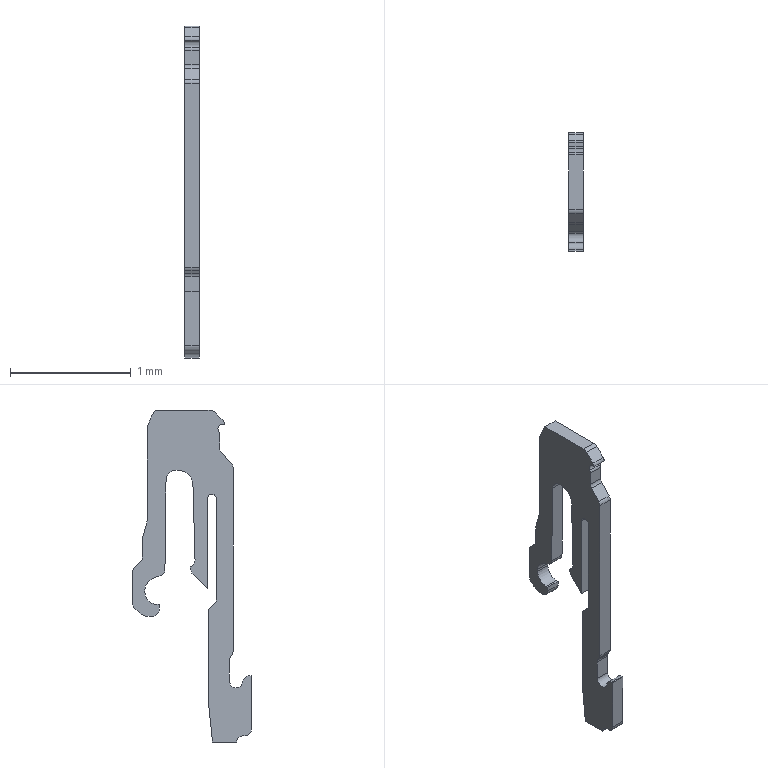Part | Creo | 1 solid | 68 faces | box 0.12 x 0.98 x 2.75 mm | volume 0.1279 mm3 | plane 38 | cylinder 30 | commonest cylinder face diameters 0.1 x14 0.08 x5 0.12 x3 0.2 x3 0.11 x1 0.14 x1